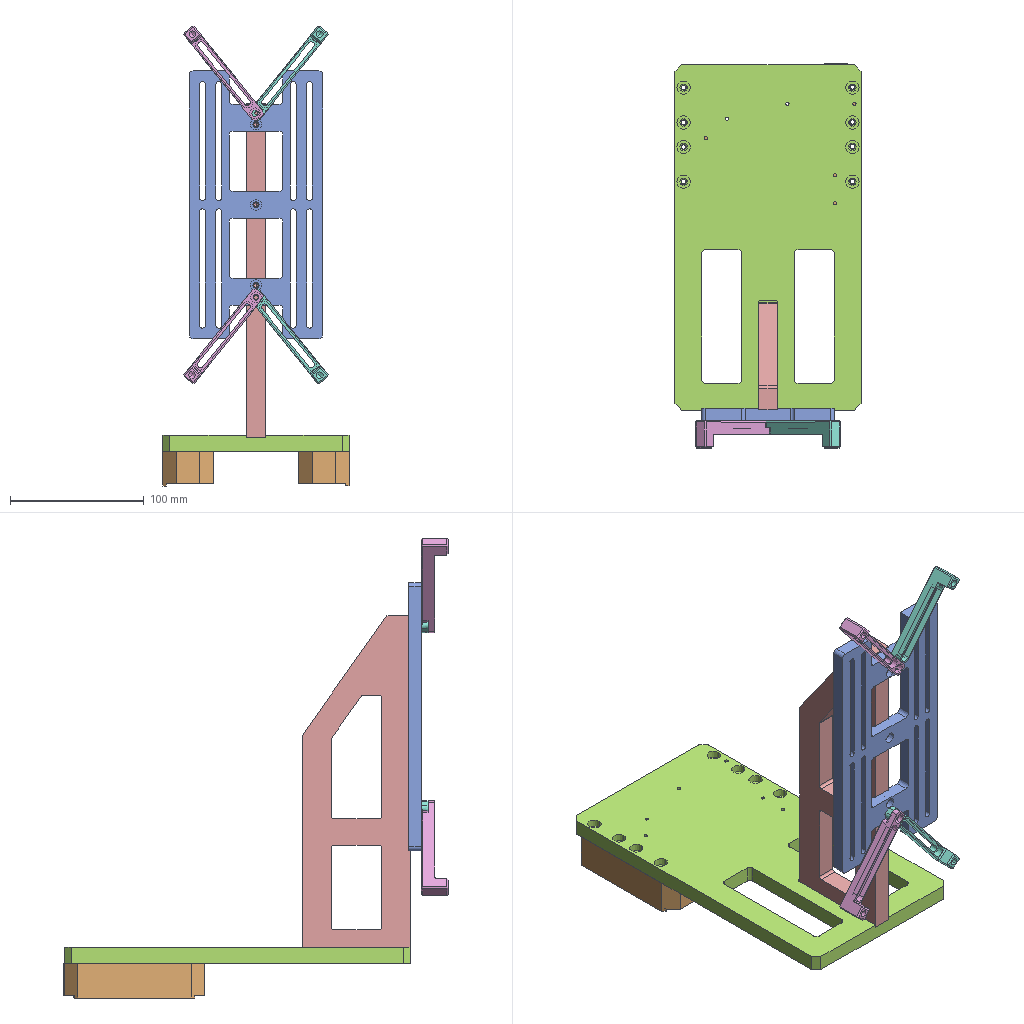Assembly | SolidWorks | 6 different items | 9 placed | box 139 x 287 x 344 mm
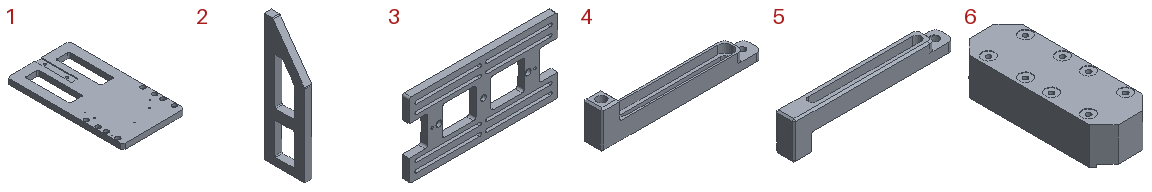Parts list (item | quantity | size | volume | features):
1 | x1 | 139 x 258 x 12 mm | 349365 mm3 | features HoleWzd 4, Cut 2, Fillet 2, Chamfer 1, Extrusion 1
2 | x1 | 14 x 80 x 250 mm | 162900 mm3 | features Fillet 3, Cut 2, HoleWzd 2, Extrusion 1
3 | x1 | 200 x 9.4 x 100 mm | 91382 mm3 | features ICE 5, Fillet 3, MirrorPattern 3, HoleWzd 2, Extrusion 1
4 | x2 | 85 x 10 x 20 mm | 4731 mm3 | features ICE 4, Chamfer 3, Fillet 3, HoleWzd 2, Extrusion 1
5 | x2 | 85 x 10 x 20 mm | 4776 mm3 | features ICE 4, Fillet 2, HoleWzd 2, Chamfer 1, Extrusion 1
6 | x2 | 37.5 x 104.657 x 26 mm | 87866 mm3 | features Chamfer 1, Cut 1, Extrusion 1, HoleWzd 1
Mates (type | each side: item.copy, entity, surface, feature):
DistanceDim | 3.1 face plane Mirror1 | 2.1 face plane Boss-Extrude1
Width | 3.1 face plane Boss-Extrude1 | 3.1 face plane Boss-Extrude1 | 2.1 face plane Boss-Extrude1 | 2.1 face plane Boss-Extrude1
Coincident | 2.1 face plane Boss-Extrude1 | 3.1 face plane Cut-Extrude5
Coincident | 3.1 face plane Boss-Extrude1 | 4.1 face plane Boss-Extrude1
Concentric | 3.1 face cylinder M4 Tapped Hole1 | 4.1 face cylinder M4 Tapped Hole1
Coincident | 4.1 face plane Cut-Extrude3 | 5.1 face plane Cut-Extrude3
Concentric | 4.1 face cylinder M4 Tapped Hole1 | 5.1 face cylinder CBORE for M4 Hexagon socket head cap screws1